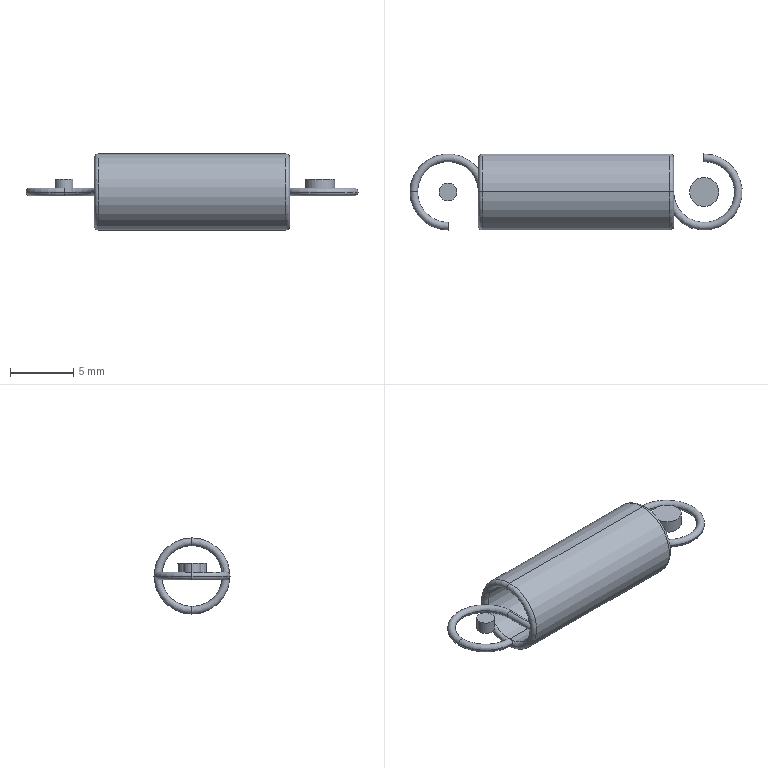Part | STEP file | 11-AWY6_2511 | 3 solids | 28 faces | box 26.2 x 6 x 6 mm | volume 169.712 mm3 | cylinder 12 | torus 10 | plane 6 | commonest cylinder face diameters 0.6 x4 1.401 x2 2.296 x2 4.8 x2 6 x2
STEP:
#1=CARTESIAN_POINT('',(23.748,0.,1.));
#2=VERTEX_POINT('',#1);
#3=CARTESIAN_POINT('',(21.452,0.,1.));
#4=VERTEX_POINT('',#3);
#5=CARTESIAN_POINT('',(22.6,0.,1.));
#6=DIRECTION('',(0.,0.,1.));
#7=DIRECTION('',(1.,0.,0.));
#8=AXIS2_PLACEMENT_3D('',#5,#6,#7);
#9=CIRCLE('',#8,1.148);
#10=EDGE_CURVE('',#2,#4,#9,.T.);
#11=ORIENTED_EDGE('',*,*,#10,.F.);
#12=CARTESIAN_POINT('',(23.748,0.,0.));
#13=VERTEX_POINT('',#12);
#14=CARTESIAN_POINT('',(23.748,0.,1.));
#15=DIRECTION('',(0.,0.,-1.));
#16=VECTOR('',#15,1000.);
#17=LINE('',#14,#16);
#18=EDGE_CURVE('',#2,#13,#17,.T.);
#19=ORIENTED_EDGE('',*,*,#18,.T.);
#20=CARTESIAN_POINT('',(21.452,0.,0.));
#21=VERTEX_POINT('',#20);
#22=CARTESIAN_POINT('',(22.6,0.,0.));
#23=DIRECTION('',(0.,0.,1.));
#24=DIRECTION('',(1.,0.,0.));
#25=AXIS2_PLACEMENT_3D('',#22,#23,#24);
#26=CIRCLE('',#25,1.148);
#27=EDGE_CURVE('',#13,#21,#26,.T.);
#28=ORIENTED_EDGE('',*,*,#27,.T.);
#29=CARTESIAN_POINT('',(21.452,0.,1.));
#30=DIRECTION('',(0.,0.,-1.));
#31=VECTOR('',#30,1000.);
#32=LINE('',#29,#31);
#33=EDGE_CURVE('',#4,#21,#32,.T.);
#34=ORIENTED_EDGE('',*,*,#33,.F.);
#35=EDGE_LOOP('',(#11,#19,#28,#34));
#36=FACE_OUTER_BOUND('',#35,.T.);
#37=CARTESIAN_POINT('',(22.6,0.,1.));
#38=DIRECTION('',(0.,0.,-1.));
#39=DIRECTION('',(-1.,0.,0.));
#40=AXIS2_PLACEMENT_3D('',#37,#38,#39);
#41=CYLINDRICAL_SURFACE('',#40,1.148);
#42=ADVANCED_FACE('',(#36),#41,.T.);
#43=ORIENTED_EDGE('',*,*,#18,.F.);
#44=CARTESIAN_POINT('',(22.6,0.,1.));
#45=DIRECTION('',(0.,0.,1.));
#46=DIRECTION('',(1.,0.,0.));
#47=AXIS2_PLACEMENT_3D('',#44,#45,#46);
#48=CIRCLE('',#47,1.148);
#49=EDGE_CURVE('',#4,#2,#48,.T.);
#50=ORIENTED_EDGE('',*,*,#49,.F.);
#51=ORIENTED_EDGE('',*,*,#33,.T.);
#52=CARTESIAN_POINT('',(22.6,0.,0.));
#53=DIRECTION('',(0.,0.,1.));
#54=DIRECTION('',(1.,0.,0.));
#55=AXIS2_PLACEMENT_3D('',#52,#53,#54);
#56=CIRCLE('',#55,1.148);
#57=EDGE_CURVE('',#21,#13,#56,.T.);
#58=ORIENTED_EDGE('',*,*,#57,.T.);
#59=EDGE_LOOP('',(#43,#50,#51,#58));
#60=FACE_OUTER_BOUND('',#59,.T.);
#61=CARTESIAN_POINT('',(22.6,0.,1.));
#62=DIRECTION('',(0.,0.,-1.));
#63=DIRECTION('',(-1.,0.,0.));
#64=AXIS2_PLACEMENT_3D('',#61,#62,#63);
#65=CYLINDRICAL_SURFACE('',#64,1.148);
#66=ADVANCED_FACE('',(#60),#65,.T.);
#67=ORIENTED_EDGE('',*,*,#49,.T.);
#68=ORIENTED_EDGE('',*,*,#10,.T.);
#69=EDGE_LOOP('',(#67,#68));
#70=FACE_OUTER_BOUND('',#69,.T.);
#71=CARTESIAN_POINT('',(22.6,0.,1.));
#72=DIRECTION('',(0.,0.,1.));
#73=DIRECTION('',(1.,0.,0.));
#74=AXIS2_PLACEMENT_3D('',#71,#72,#73);
#75=PLANE('',#74);
#76=ADVANCED_FACE('',(#70),#75,.T.);
#77=ORIENTED_EDGE('',*,*,#57,.F.);
#78=ORIENTED_EDGE('',*,*,#27,.F.);
#79=EDGE_LOOP('',(#77,#78));
#80=FACE_OUTER_BOUND('',#79,.T.);
#81=CARTESIAN_POINT('',(22.6,0.,0.));
#82=DIRECTION('',(0.,0.,1.));
#83=DIRECTION('',(1.,0.,0.));
#84=AXIS2_PLACEMENT_3D('',#81,#82,#83);
#85=PLANE('',#84);
#86=ADVANCED_FACE('',(#80),#85,.F.);
#87=CLOSED_SHELL('',(#42,#66,#76,#86));
#88=MANIFOLD_SOLID_BREP('',#87);
#89=CARTESIAN_POINT('',(3.1,0.,1.));
#90=VERTEX_POINT('',#89);
#91=CARTESIAN_POINT('',(1.7,0.,1.));
#92=VERTEX_POINT('',#91);
#93=CARTESIAN_POINT('',(2.4,0.,1.));
#94=DIRECTION('',(0.,0.,1.));
#95=DIRECTION('',(1.,0.,0.));
#96=AXIS2_PLACEMENT_3D('',#93,#94,#95);
#97=CIRCLE('',#96,0.7003);
#98=EDGE_CURVE('',#90,#92,#97,.T.);
#99=ORIENTED_EDGE('',*,*,#98,.F.);
#100=CARTESIAN_POINT('',(3.1,0.,0.));
#101=VERTEX_POINT('',#100);
#102=CARTESIAN_POINT('',(3.1,0.,1.));
#103=DIRECTION('',(0.,0.,-1.));
#104=VECTOR('',#103,1000.);
#105=LINE('',#102,#104);
#106=EDGE_CURVE('',#90,#101,#105,.T.);
#107=ORIENTED_EDGE('',*,*,#106,.T.);
#108=CARTESIAN_POINT('',(1.7,0.,0.));
#109=VERTEX_POINT('',#108);
#110=CARTESIAN_POINT('',(2.4,0.,0.));
#111=DIRECTION('',(0.,0.,1.));
#112=DIRECTION('',(1.,0.,0.));
#113=AXIS2_PLACEMENT_3D('',#110,#111,#112);
#114=CIRCLE('',#113,0.7003);
#115=EDGE_CURVE('',#101,#109,#114,.T.);
#116=ORIENTED_EDGE('',*,*,#115,.T.);
#117=CARTESIAN_POINT('',(1.7,0.,1.));
#118=DIRECTION('',(0.,0.,-1.));
#119=VECTOR('',#118,1000.);
#120=LINE('',#117,#119);
#121=EDGE_CURVE('',#92,#109,#120,.T.);
#122=ORIENTED_EDGE('',*,*,#121,.F.);
#123=EDGE_LOOP('',(#99,#107,#116,#122));
#124=FACE_OUTER_BOUND('',#123,.T.);
#125=CARTESIAN_POINT('',(2.4,0.,1.));
#126=DIRECTION('',(0.,0.,-1.));
#127=DIRECTION('',(-1.,0.,0.));
#128=AXIS2_PLACEMENT_3D('',#125,#126,#127);
#129=CYLINDRICAL_SURFACE('',#128,0.7003);
#130=ADVANCED_FACE('',(#124),#129,.T.);
#131=ORIENTED_EDGE('',*,*,#106,.F.);
#132=CARTESIAN_POINT('',(2.4,0.,1.));
#133=DIRECTION('',(0.,0.,1.));
#134=DIRECTION('',(1.,0.,0.));
#135=AXIS2_PLACEMENT_3D('',#132,#133,#134);
#136=CIRCLE('',#135,0.7003);
#137=EDGE_CURVE('',#92,#90,#136,.T.);
#138=ORIENTED_EDGE('',*,*,#137,.F.);
#139=ORIENTED_EDGE('',*,*,#121,.T.);
#140=CARTESIAN_POINT('',(2.4,0.,0.));
#141=DIRECTION('',(0.,0.,1.));
#142=DIRECTION('',(1.,0.,0.));
#143=AXIS2_PLACEMENT_3D('',#140,#141,#142);
#144=CIRCLE('',#143,0.7003);
#145=EDGE_CURVE('',#109,#101,#144,.T.);
#146=ORIENTED_EDGE('',*,*,#145,.T.);
#147=EDGE_LOOP('',(#131,#138,#139,#146));
#148=FACE_OUTER_BOUND('',#147,.T.);
#149=CARTESIAN_POINT('',(2.4,0.,1.));
#150=DIRECTION('',(0.,0.,-1.));
#151=DIRECTION('',(-1.,0.,0.));
#152=AXIS2_PLACEMENT_3D('',#149,#150,#151);
#153=CYLINDRICAL_SURFACE('',#152,0.7003);
#154=ADVANCED_FACE('',(#148),#153,.T.);
#155=ORIENTED_EDGE('',*,*,#137,.T.);
#156=ORIENTED_EDGE('',*,*,#98,.T.);
#157=EDGE_LOOP('',(#155,#156));
#158=FACE_OUTER_BOUND('',#157,.T.);
#159=CARTESIAN_POINT('',(2.4,0.,1.));
#160=DIRECTION('',(0.,0.,1.));
#161=DIRECTION('',(1.,0.,0.));
#162=AXIS2_PLACEMENT_3D('',#159,#160,#161);
#163=PLANE('',#162);
#164=ADVANCED_FACE('',(#158),#163,.T.);
#165=ORIENTED_EDGE('',*,*,#145,.F.);
#166=ORIENTED_EDGE('',*,*,#115,.F.);
#167=EDGE_LOOP('',(#165,#166));
#168=FACE_OUTER_BOUND('',#167,.T.);
#169=CARTESIAN_POINT('',(2.4,0.,0.));
#170=DIRECTION('',(0.,0.,1.));
#171=DIRECTION('',(1.,0.,0.));
#172=AXIS2_PLACEMENT_3D('',#169,#170,#171);
#173=PLANE('',#172);
#174=ADVANCED_FACE('',(#168),#173,.F.);
#175=CLOSED_SHELL('',(#130,#154,#164,#174));
#176=MANIFOLD_SOLID_BREP('',#175);
#177=CARTESIAN_POINT('',(-0.6,0.,0.));
#178=VERTEX_POINT('',#177);
#179=CARTESIAN_POINT('',(0.,0.,0.));
#180=VERTEX_POINT('',#179);
#181=CARTESIAN_POINT('',(-0.3,0.,0.));
#182=DIRECTION('',(0.,-1.,0.));
#183=DIRECTION('',(0.,0.,-1.));
#184=AXIS2_PLACEMENT_3D('',#181,#182,#183);
#185=CIRCLE('',#184,0.3);
#186=EDGE_CURVE('',#178,#180,#185,.T.);
#187=ORIENTED_EDGE('',*,*,#186,.F.);
#188=CARTESIAN_POINT('',(5.4,0.,0.));
#189=VERTEX_POINT('',#188);
#190=CARTESIAN_POINT('',(2.4,0.,0.));
#191=DIRECTION('',(0.,0.,-1.));
#192=DIRECTION('',(-1.,0.,0.));
#193=AXIS2_PLACEMENT_3D('',#190,#191,#192);
#194=CIRCLE('',#193,3.);
#195=EDGE_CURVE('',#178,#189,#194,.T.);
#196=ORIENTED_EDGE('',*,*,#195,.T.);
#197=CARTESIAN_POINT('',(5.1,0.,-0.3));
#198=VERTEX_POINT('',#197);
#199=CARTESIAN_POINT('',(5.1,0.,0.));
#200=DIRECTION('',(0.,-1.,0.));
#201=DIRECTION('',(0.,0.,-1.));
#202=AXIS2_PLACEMENT_3D('',#199,#200,#201);
#203=CIRCLE('',#202,0.3);
#204=EDGE_CURVE('',#198,#189,#203,.T.);
#205=ORIENTED_EDGE('',*,*,#204,.F.);
#206=CARTESIAN_POINT('',(4.8,0.,0.));
#207=VERTEX_POINT('',#206);
#208=CARTESIAN_POINT('',(5.1,0.,0.));
#209=DIRECTION('',(0.,-1.,0.));
#210=DIRECTION('',(0.,0.,-1.));
#211=AXIS2_PLACEMENT_3D('',#208,#209,#210);
#212=CIRCLE('',#211,0.3);
#213=EDGE_CURVE('',#207,#198,#212,.T.);
#214=ORIENTED_EDGE('',*,*,#213,.F.);
#215=CARTESIAN_POINT('',(2.4,0.,0.));
#216=DIRECTION('',(0.,0.,-1.));
#217=DIRECTION('',(-1.,0.,0.));
#218=AXIS2_PLACEMENT_3D('',#215,#216,#217);
#219=CIRCLE('',#218,2.4);
#220=EDGE_CURVE('',#180,#207,#219,.T.);
#221=ORIENTED_EDGE('',*,*,#220,.F.);
#222=EDGE_LOOP('',(#187,#196,#205,#214,#221));
#223=FACE_OUTER_BOUND('',#222,.T.);
#224=CARTESIAN_POINT('',(2.4,0.,0.));
#225=DIRECTION('',(0.,0.,-1.));
#226=DIRECTION('',(-1.,0.,0.));
#227=AXIS2_PLACEMENT_3D('',#224,#225,#226);
#228=TOROIDAL_SURFACE('',#227,2.7,0.3);
#229=ADVANCED_FACE('',(#223),#228,.T.);
#230=CARTESIAN_POINT('',(22.558,2.4,0.));
#231=VERTEX_POINT('',#230);
#232=CARTESIAN_POINT('',(22.548,3.,0.));
#233=VERTEX_POINT('',#232);
#234=CARTESIAN_POINT('',(22.553,2.7,0.));
#235=DIRECTION('',(0.9998,0.01745,0.));
#236=DIRECTION('',(0.,0.,1.));
#237=AXIS2_PLACEMENT_3D('',#234,#235,#236);
#238=CIRCLE('',#237,0.3);
#239=EDGE_CURVE('',#231,#233,#238,.T.);
#240=ORIENTED_EDGE('',*,*,#239,.T.);
#241=CARTESIAN_POINT('',(19.6,0.,0.));
#242=VERTEX_POINT('',#241);
#243=CARTESIAN_POINT('',(22.6,0.,0.));
#244=DIRECTION('',(0.,0.,-1.));
#245=DIRECTION('',(-1.,0.,0.));
#246=AXIS2_PLACEMENT_3D('',#243,#244,#245);
#247=CIRCLE('',#246,3.);
#248=EDGE_CURVE('',#233,#242,#247,.T.);
#249=ORIENTED_EDGE('',*,*,#248,.T.);
#250=CARTESIAN_POINT('',(19.9,0.,-0.3));
#251=VERTEX_POINT('',#250);
#252=CARTESIAN_POINT('',(19.9,0.,0.));
#253=DIRECTION('',(0.,1.,0.));
#254=DIRECTION('',(0.,0.,1.));
#255=AXIS2_PLACEMENT_3D('',#252,#253,#254);
#256=CIRCLE('',#255,0.3);
#257=EDGE_CURVE('',#251,#242,#256,.T.);
#258=ORIENTED_EDGE('',*,*,#257,.F.);
#259=CARTESIAN_POINT('',(20.2,0.,0.));
#260=VERTEX_POINT('',#259);
#261=CARTESIAN_POINT('',(19.9,0.,0.));
#262=DIRECTION('',(0.,1.,0.));
#263=DIRECTION('',(0.,0.,1.));
#264=AXIS2_PLACEMENT_3D('',#261,#262,#263);
#265=CIRCLE('',#264,0.3);
#266=EDGE_CURVE('',#260,#251,#265,.T.);
#267=ORIENTED_EDGE('',*,*,#266,.F.);
#268=CARTESIAN_POINT('',(22.6,0.,0.));
#269=DIRECTION('',(0.,0.,-1.));
#270=DIRECTION('',(-1.,0.,0.));
#271=AXIS2_PLACEMENT_3D('',#268,#269,#270);
#272=CIRCLE('',#271,2.4);
#273=EDGE_CURVE('',#231,#260,#272,.T.);
#274=ORIENTED_EDGE('',*,*,#273,.F.);
#275=EDGE_LOOP('',(#240,#249,#258,#267,#274));
#276=FACE_OUTER_BOUND('',#275,.T.);
#277=CARTESIAN_POINT('',(22.6,0.,0.));
#278=DIRECTION('',(0.,0.,-1.));
#279=DIRECTION('',(-1.,0.,0.));
#280=AXIS2_PLACEMENT_3D('',#277,#278,#279);
#281=TOROIDAL_SURFACE('',#280,2.7,0.3);
#282=ADVANCED_FACE('',(#276),#281,.T.);
#283=CARTESIAN_POINT('',(2.452,-3.,0.));
#284=VERTEX_POINT('',#283);
#285=CARTESIAN_POINT('',(2.442,-2.4,0.));
#286=VERTEX_POINT('',#285);
#287=CARTESIAN_POINT('',(2.447,-2.7,0.));
#288=DIRECTION('',(0.9998,0.01745,0.));
#289=DIRECTION('',(0.,0.,1.));
#290=AXIS2_PLACEMENT_3D('',#287,#288,#289);
#291=CIRCLE('',#290,0.3);
#292=EDGE_CURVE('',#284,#286,#291,.T.);
#293=ORIENTED_EDGE('',*,*,#292,.F.);
#294=CARTESIAN_POINT('',(2.4,0.,0.));
#295=DIRECTION('',(0.,0.,-1.));
#296=DIRECTION('',(-1.,0.,0.));
#297=AXIS2_PLACEMENT_3D('',#294,#295,#296);
#298=CIRCLE('',#297,3.);
#299=EDGE_CURVE('',#284,#178,#298,.T.);
#300=ORIENTED_EDGE('',*,*,#299,.T.);
#301=ORIENTED_EDGE('',*,*,#186,.T.);
#302=CARTESIAN_POINT('',(2.4,0.,0.));
#303=DIRECTION('',(0.,0.,-1.));
#304=DIRECTION('',(-1.,0.,0.));
#305=AXIS2_PLACEMENT_3D('',#302,#303,#304);
#306=CIRCLE('',#305,2.4);
#307=EDGE_CURVE('',#286,#180,#306,.T.);
#308=ORIENTED_EDGE('',*,*,#307,.F.);
#309=EDGE_LOOP('',(#293,#300,#301,#308));
#310=FACE_OUTER_BOUND('',#309,.T.);
#311=CARTESIAN_POINT('',(2.4,0.,0.));
#312=DIRECTION('',(0.,0.,-1.));
#313=DIRECTION('',(-1.,0.,0.));
#314=AXIS2_PLACEMENT_3D('',#311,#312,#313);
#315=TOROIDAL_SURFACE('',#314,2.7,0.3);
#316=ADVANCED_FACE('',(#310),#315,.T.);
#317=ORIENTED_EDGE('',*,*,#299,.F.);
#318=CARTESIAN_POINT('',(2.447,-2.7,0.));
#319=DIRECTION('',(0.9998,0.01745,0.));
#320=DIRECTION('',(0.,0.,1.));
#321=AXIS2_PLACEMENT_3D('',#318,#319,#320);
#322=CIRCLE('',#321,0.3);
#323=EDGE_CURVE('',#286,#284,#322,.T.);
#324=ORIENTED_EDGE('',*,*,#323,.F.);
#325=ORIENTED_EDGE('',*,*,#307,.T.);
#326=CARTESIAN_POINT('',(-0.3,0.,0.));
#327=DIRECTION('',(0.,-1.,0.));
#328=DIRECTION('',(0.,0.,-1.));
#329=AXIS2_PLACEMENT_3D('',#326,#327,#328);
#330=CIRCLE('',#329,0.3);
#331=EDGE_CURVE('',#180,#178,#330,.T.);
#332=ORIENTED_EDGE('',*,*,#331,.T.);
#333=EDGE_LOOP('',(#317,#324,#325,#332));
#334=FACE_OUTER_BOUND('',#333,.T.);
#335=CARTESIAN_POINT('',(2.4,0.,0.));
#336=DIRECTION('',(0.,0.,-1.));
#337=DIRECTION('',(-1.,0.,0.));
#338=AXIS2_PLACEMENT_3D('',#335,#336,#337);
#339=TOROIDAL_SURFACE('',#338,2.7,0.3);
#340=ADVANCED_FACE('',(#334),#339,.T.);
#341=ORIENTED_EDGE('',*,*,#204,.T.);
#342=CARTESIAN_POINT('',(5.1,0.,0.3));
#343=VERTEX_POINT('',#342);
#344=CARTESIAN_POINT('',(5.1,0.,0.));
#345=DIRECTION('',(0.,-1.,0.));
#346=DIRECTION('',(0.,0.,-1.));
#347=AXIS2_PLACEMENT_3D('',#344,#345,#346);
#348=CIRCLE('',#347,0.3);
#349=EDGE_CURVE('',#189,#343,#348,.T.);
#350=ORIENTED_EDGE('',*,*,#349,.T.);
#351=CARTESIAN_POINT('',(5.1,-2.381,0.3));
#352=VERTEX_POINT('',#351);
#353=CARTESIAN_POINT('',(5.1,-2.7,0.3));
#354=DIRECTION('',(0.,-1.,0.));
#355=VECTOR('',#354,1000.);
#356=LINE('',#353,#355);
#357=EDGE_CURVE('',#343,#352,#356,.T.);
#358=ORIENTED_EDGE('',*,*,#357,.T.);
#359=CARTESIAN_POINT('',(5.1,-2.381,-0.3));
#360=VERTEX_POINT('',#359);
#361=CARTESIAN_POINT('',(5.1,-2.381,-0.3));
#362=CARTESIAN_POINT('',(5.179,-2.381,-0.3));
#363=CARTESIAN_POINT('',(5.257,-2.386,-0.2674));
#364=CARTESIAN_POINT('',(5.367,-2.396,-0.1568));
#365=CARTESIAN_POINT('',(5.4,-2.4,-0.07846));
#366=CARTESIAN_POINT('',(5.4,-2.4,0.07824));
#367=CARTESIAN_POINT('',(5.368,-2.396,0.1561));
#368=CARTESIAN_POINT('',(5.256,-2.386,0.2681));
#369=CARTESIAN_POINT('',(5.178,-2.381,0.3));
#370=CARTESIAN_POINT('',(5.1,-2.381,0.3));
#371=B_SPLINE_CURVE_WITH_KNOTS('',3,(#361,#362,#363,#364,#365,#366,#367,#368,#369,#370),.UNSPECIFIED.,.F.,.F.,(4,2,2,2,4),(0.,0.0002347,0.0004694,0.0007041,0.0009389),.UNSPECIFIED.);
#372=EDGE_CURVE('',#360,#352,#371,.T.);
#373=ORIENTED_EDGE('',*,*,#372,.F.);
#374=CARTESIAN_POINT('',(5.1,-2.7,-0.3));
#375=DIRECTION('',(0.,-1.,0.));
#376=VECTOR('',#375,1000.);
#377=LINE('',#374,#376);
#378=EDGE_CURVE('',#198,#360,#377,.T.);
#379=ORIENTED_EDGE('',*,*,#378,.F.);
#380=EDGE_LOOP('',(#341,#350,#358,#373,#379));
#381=FACE_OUTER_BOUND('',#380,.T.);
#382=CARTESIAN_POINT('',(5.1,-2.7,0.));
#383=DIRECTION('',(0.,-1.,0.));
#384=DIRECTION('',(0.,0.,-1.));
#385=AXIS2_PLACEMENT_3D('',#382,#383,#384);
#386=CYLINDRICAL_SURFACE('',#385,0.3);
#387=ADVANCED_FACE('',(#381),#386,.T.);
#388=CARTESIAN_POINT('',(19.9,0.,0.3));
#389=VERTEX_POINT('',#388);
#390=CARTESIAN_POINT('',(19.9,0.,0.));
#391=DIRECTION('',(0.,1.,0.));
#392=DIRECTION('',(0.,0.,1.));
#393=AXIS2_PLACEMENT_3D('',#390,#391,#392);
#394=CIRCLE('',#393,0.3);
#395=EDGE_CURVE('',#389,#260,#394,.T.);
#396=ORIENTED_EDGE('',*,*,#395,.T.);
#397=ORIENTED_EDGE('',*,*,#266,.T.);
#398=CARTESIAN_POINT('',(19.9,2.381,-0.3));
#399=VERTEX_POINT('',#398);
#400=CARTESIAN_POINT('',(19.9,0.,-0.3));
#401=DIRECTION('',(0.,1.,0.));
#402=VECTOR('',#401,1000.);
#403=LINE('',#400,#402);
#404=EDGE_CURVE('',#251,#399,#403,.T.);
#405=ORIENTED_EDGE('',*,*,#404,.T.);
#406=CARTESIAN_POINT('',(20.2,2.7,0.));
#407=VERTEX_POINT('',#406);
#408=CARTESIAN_POINT('',(19.9,2.381,-0.3));
#409=CARTESIAN_POINT('',(19.949,2.381,-0.3));
#410=CARTESIAN_POINT('',(19.996,2.395,-0.2875));
#411=CARTESIAN_POINT('',(20.074,2.439,-0.2481));
#412=CARTESIAN_POINT('',(20.105,2.468,-0.2221));
#413=CARTESIAN_POINT('',(20.178,2.561,-0.1362));
#414=CARTESIAN_POINT('',(20.2,2.632,-0.06843));
#415=CARTESIAN_POINT('',(20.2,2.7,0.));
#416=B_SPLINE_CURVE_WITH_KNOTS('',3,(#408,#409,#410,#411,#412,#413,#414,#415),.UNSPECIFIED.,.F.,.F.,(4,2,2,4),(0.000000196,0.0001454,0.0002906,0.000581),.UNSPECIFIED.);
#417=EDGE_CURVE('',#399,#407,#416,.T.);
#418=ORIENTED_EDGE('',*,*,#417,.T.);
#419=CARTESIAN_POINT('',(19.9,2.381,0.3));
#420=VERTEX_POINT('',#419);
#421=CARTESIAN_POINT('',(20.2,2.7,0.));
#422=CARTESIAN_POINT('',(20.2,2.632,0.0681));
#423=CARTESIAN_POINT('',(20.178,2.561,0.1362));
#424=CARTESIAN_POINT('',(20.105,2.468,0.2218));
#425=CARTESIAN_POINT('',(20.074,2.44,0.2479));
#426=CARTESIAN_POINT('',(19.997,2.396,0.2873));
#427=CARTESIAN_POINT('',(19.949,2.381,0.3));
#428=CARTESIAN_POINT('',(19.9,2.381,0.3));
#429=B_SPLINE_CURVE_WITH_KNOTS('',3,(#421,#422,#423,#424,#425,#426,#427,#428),.UNSPECIFIED.,.F.,.F.,(4,2,2,4),(-0.000003464,0.0002855,0.00043,0.0005745),.UNSPECIFIED.);
#430=EDGE_CURVE('',#407,#420,#429,.T.);
#431=ORIENTED_EDGE('',*,*,#430,.T.);
#432=CARTESIAN_POINT('',(19.9,0.,0.3));
#433=DIRECTION('',(0.,1.,0.));
#434=VECTOR('',#433,1000.);
#435=LINE('',#432,#434);
#436=EDGE_CURVE('',#389,#420,#435,.T.);
#437=ORIENTED_EDGE('',*,*,#436,.F.);
#438=EDGE_LOOP('',(#396,#397,#405,#418,#431,#437));
#439=FACE_OUTER_BOUND('',#438,.T.);
#440=CARTESIAN_POINT('',(19.9,0.,0.));
#441=DIRECTION('',(0.,1.,0.));
#442=DIRECTION('',(0.,0.,1.));
#443=AXIS2_PLACEMENT_3D('',#440,#441,#442);
#444=CYLINDRICAL_SURFACE('',#443,0.3);
#445=ADVANCED_FACE('',(#439),#444,.T.);
#446=CARTESIAN_POINT('',(19.9,0.,3.));
#447=VERTEX_POINT('',#446);
#448=CARTESIAN_POINT('',(19.9,0.,-3.));
#449=VERTEX_POINT('',#448);
#450=CARTESIAN_POINT('',(19.9,0.,0.));
#451=DIRECTION('',(-1.,0.,0.));
#452=DIRECTION('',(0.,0.,1.));
#453=AXIS2_PLACEMENT_3D('',#450,#451,#452);
#454=CIRCLE('',#453,3.);
#455=EDGE_CURVE('',#447,#449,#454,.T.);
#456=ORIENTED_EDGE('',*,*,#455,.T.);
#457=CARTESIAN_POINT('',(5.1,0.,-3.));
#458=VERTEX_POINT('',#457);
#459=CARTESIAN_POINT('',(20.2,0.,-3.));
#460=DIRECTION('',(-1.,0.,0.));
#461=VECTOR('',#460,1000.);
#462=LINE('',#459,#461);
#463=EDGE_CURVE('',#449,#458,#462,.T.);
#464=ORIENTED_EDGE('',*,*,#463,.T.);
#465=CARTESIAN_POINT('',(5.1,0.,3.));
#466=VERTEX_POINT('',#465);
#467=CARTESIAN_POINT('',(5.1,0.,0.));
#468=DIRECTION('',(-1.,0.,0.));
#469=DIRECTION('',(0.,0.,1.));
#470=AXIS2_PLACEMENT_3D('',#467,#468,#469);
#471=CIRCLE('',#470,3.);
#472=EDGE_CURVE('',#466,#458,#471,.T.);
#473=ORIENTED_EDGE('',*,*,#472,.F.);
#474=CARTESIAN_POINT('',(20.2,0.,3.));
#475=DIRECTION('',(-1.,0.,0.));
#476=VECTOR('',#475,1000.);
#477=LINE('',#474,#476);
#478=EDGE_CURVE('',#447,#466,#477,.T.);
#479=ORIENTED_EDGE('',*,*,#478,.F.);
#480=EDGE_LOOP('',(#456,#464,#473,#479));
#481=FACE_OUTER_BOUND('',#480,.T.);
#482=CARTESIAN_POINT('',(20.2,0.,0.));
#483=DIRECTION('',(-1.,0.,0.));
#484=DIRECTION('',(0.,0.,1.));
#485=AXIS2_PLACEMENT_3D('',#482,#483,#484);
#486=CYLINDRICAL_SURFACE('',#485,3.);
#487=ADVANCED_FACE('',(#481),#486,.T.);
#488=ORIENTED_EDGE('',*,*,#472,.T.);
#489=CARTESIAN_POINT('',(5.1,0.,-2.4));
#490=VERTEX_POINT('',#489);
#491=CARTESIAN_POINT('',(5.1,0.,-2.7));
#492=DIRECTION('',(0.,1.,0.));
#493=DIRECTION('',(0.,0.,1.));
#494=AXIS2_PLACEMENT_3D('',#491,#492,#493);
#495=CIRCLE('',#494,0.3);
#496=EDGE_CURVE('',#458,#490,#495,.T.);
#497=ORIENTED_EDGE('',*,*,#496,.T.);
#498=CARTESIAN_POINT('',(5.1,0.,2.4));
#499=VERTEX_POINT('',#498);
#500=CARTESIAN_POINT('',(5.1,0.,0.));
#501=DIRECTION('',(-1.,0.,0.));
#502=DIRECTION('',(0.,0.,1.));
#503=AXIS2_PLACEMENT_3D('',#500,#501,#502);
#504=CIRCLE('',#503,2.4);
#505=EDGE_CURVE('',#499,#490,#504,.T.);
#506=ORIENTED_EDGE('',*,*,#505,.F.);
#507=CARTESIAN_POINT('',(5.1,0.,2.7));
#508=DIRECTION('',(0.,-1.,0.));
#509=DIRECTION('',(0.,0.,-1.));
#510=AXIS2_PLACEMENT_3D('',#507,#508,#509);
#511=CIRCLE('',#510,0.3);
#512=EDGE_CURVE('',#466,#499,#511,.T.);
#513=ORIENTED_EDGE('',*,*,#512,.F.);
#514=EDGE_LOOP('',(#488,#497,#506,#513));
#515=FACE_OUTER_BOUND('',#514,.T.);
#516=CARTESIAN_POINT('',(5.1,0.,0.));
#517=DIRECTION('',(-1.,0.,0.));
#518=DIRECTION('',(0.,0.,1.));
#519=AXIS2_PLACEMENT_3D('',#516,#517,#518);
#520=TOROIDAL_SURFACE('',#519,2.7,0.3);
#521=ADVANCED_FACE('',(#515),#520,.T.);
#522=CARTESIAN_POINT('',(19.9,0.,-2.4));
#523=VERTEX_POINT('',#522);
#524=CARTESIAN_POINT('',(19.9,0.,0.));
#525=DIRECTION('',(-1.,0.,0.));
#526=DIRECTION('',(0.,0.,1.));
#527=AXIS2_PLACEMENT_3D('',#524,#525,#526);
#528=CIRCLE('',#527,2.4);
#529=EDGE_CURVE('',#399,#523,#528,.T.);
#530=ORIENTED_EDGE('',*,*,#529,.T.);
#531=CARTESIAN_POINT('',(19.9,0.,-2.7));
#532=DIRECTION('',(0.,1.,0.));
#533=DIRECTION('',(0.,0.,1.));
#534=AXIS2_PLACEMENT_3D('',#531,#532,#533);
#535=CIRCLE('',#534,0.3);
#536=EDGE_CURVE('',#523,#449,#535,.T.);
#537=ORIENTED_EDGE('',*,*,#536,.T.);
#538=ORIENTED_EDGE('',*,*,#455,.F.);
#539=CARTESIAN_POINT('',(19.9,0.,2.4));
#540=VERTEX_POINT('',#539);
#541=CARTESIAN_POINT('',(19.9,0.,2.7));
#542=DIRECTION('',(0.,-1.,0.));
#543=DIRECTION('',(0.,0.,-1.));
#544=AXIS2_PLACEMENT_3D('',#541,#542,#543);
#545=CIRCLE('',#544,0.3);
#546=EDGE_CURVE('',#540,#447,#545,.T.);
#547=ORIENTED_EDGE('',*,*,#546,.F.);
#548=CARTESIAN_POINT('',(19.9,0.,0.));
#549=DIRECTION('',(-1.,0.,0.));
#550=DIRECTION('',(0.,0.,1.));
#551=AXIS2_PLACEMENT_3D('',#548,#549,#550);
#552=CIRCLE('',#551,2.4);
#553=EDGE_CURVE('',#540,#420,#552,.T.);
#554=ORIENTED_EDGE('',*,*,#553,.T.);
#555=ORIENTED_EDGE('',*,*,#430,.F.);
#556=ORIENTED_EDGE('',*,*,#417,.F.);
#557=EDGE_LOOP('',(#530,#537,#538,#547,#554,#555,#556));
#558=FACE_OUTER_BOUND('',#557,.T.);
#559=CARTESIAN_POINT('',(19.9,0.,0.));
#560=DIRECTION('',(-1.,0.,0.));
#561=DIRECTION('',(0.,0.,1.));
#562=AXIS2_PLACEMENT_3D('',#559,#560,#561);
#563=TOROIDAL_SURFACE('',#562,2.7,0.3);
#564=ADVANCED_FACE('',(#558),#563,.T.);
#565=CARTESIAN_POINT('',(19.9,0.,0.));
#566=DIRECTION('',(-1.,0.,0.));
#567=DIRECTION('',(0.,0.,1.));
#568=AXIS2_PLACEMENT_3D('',#565,#566,#567);
#569=CIRCLE('',#568,2.4);
#570=EDGE_CURVE('',#523,#540,#569,.T.);
#571=ORIENTED_EDGE('',*,*,#570,.F.);
#572=CARTESIAN_POINT('',(20.2,0.,-2.4));
#573=DIRECTION('',(-1.,0.,0.));
#574=VECTOR('',#573,1000.);
#575=LINE('',#572,#574);
#576=EDGE_CURVE('',#523,#490,#575,.T.);
#577=ORIENTED_EDGE('',*,*,#576,.T.);
#578=CARTESIAN_POINT('',(5.1,0.,0.));
#579=DIRECTION('',(-1.,0.,0.));
#580=DIRECTION('',(0.,0.,1.));
#581=AXIS2_PLACEMENT_3D('',#578,#579,#580);
#582=CIRCLE('',#581,2.4);
#583=EDGE_CURVE('',#490,#360,#582,.T.);
#584=ORIENTED_EDGE('',*,*,#583,.T.);
#585=ORIENTED_EDGE('',*,*,#372,.T.);
#586=CARTESIAN_POINT('',(5.1,0.,0.));
#587=DIRECTION('',(-1.,0.,0.));
#588=DIRECTION('',(0.,0.,1.));
#589=AXIS2_PLACEMENT_3D('',#586,#587,#588);
#590=CIRCLE('',#589,2.4);
#591=EDGE_CURVE('',#352,#499,#590,.T.);
#592=ORIENTED_EDGE('',*,*,#591,.T.);
#593=CARTESIAN_POINT('',(20.2,0.,2.4));
#594=DIRECTION('',(-1.,0.,0.));
#595=VECTOR('',#594,1000.);
#596=LINE('',#593,#595);
#597=EDGE_CURVE('',#540,#499,#596,.T.);
#598=ORIENTED_EDGE('',*,*,#597,.F.);
#599=EDGE_LOOP('',(#571,#577,#584,#585,#592,#598));
#600=FACE_OUTER_BOUND('',#599,.T.);
#601=CARTESIAN_POINT('',(20.2,0.,0.));
#602=DIRECTION('',(-1.,0.,0.));
#603=DIRECTION('',(0.,0.,1.));
#604=AXIS2_PLACEMENT_3D('',#601,#602,#603);
#605=CYLINDRICAL_SURFACE('',#604,2.4);
#606=ADVANCED_FACE('',(#600),#605,.F.);
#607=ORIENTED_EDGE('',*,*,#576,.F.);
#608=ORIENTED_EDGE('',*,*,#529,.F.);
#609=CARTESIAN_POINT('',(19.9,2.381,0.3));
#610=CARTESIAN_POINT('',(19.821,2.381,0.3));
#611=CARTESIAN_POINT('',(19.743,2.386,0.2674));
#612=CARTESIAN_POINT('',(19.633,2.396,0.1568));
#613=CARTESIAN_POINT('',(19.6,2.4,0.07846));
#614=CARTESIAN_POINT('',(19.6,2.4,-0.07824));
#615=CARTESIAN_POINT('',(19.632,2.396,-0.1561));
#616=CARTESIAN_POINT('',(19.744,2.386,-0.2681));
#617=CARTESIAN_POINT('',(19.822,2.381,-0.3));
#618=CARTESIAN_POINT('',(19.9,2.381,-0.3));
#619=B_SPLINE_CURVE_WITH_KNOTS('',3,(#609,#610,#611,#612,#613,#614,#615,#616,#617,#618),.UNSPECIFIED.,.F.,.F.,(4,2,2,2,4),(0.,0.0002347,0.0004694,0.0007041,0.0009389),.UNSPECIFIED.);
#620=EDGE_CURVE('',#420,#399,#619,.T.);
#621=ORIENTED_EDGE('',*,*,#620,.F.);
#622=ORIENTED_EDGE('',*,*,#553,.F.);
#623=ORIENTED_EDGE('',*,*,#597,.T.);
#624=ORIENTED_EDGE('',*,*,#505,.T.);
#625=EDGE_LOOP('',(#607,#608,#621,#622,#623,#624));
#626=FACE_OUTER_BOUND('',#625,.T.);
#627=CARTESIAN_POINT('',(20.2,0.,0.));
#628=DIRECTION('',(-1.,0.,0.));
#629=DIRECTION('',(0.,0.,1.));
#630=AXIS2_PLACEMENT_3D('',#627,#628,#629);
#631=CYLINDRICAL_SURFACE('',#630,2.4);
#632=ADVANCED_FACE('',(#626),#631,.F.);
#633=ORIENTED_EDGE('',*,*,#536,.F.);
#634=ORIENTED_EDGE('',*,*,#570,.T.);
#635=ORIENTED_EDGE('',*,*,#546,.T.);
#636=CARTESIAN_POINT('',(19.9,0.,0.));
#637=DIRECTION('',(-1.,0.,0.));
#638=DIRECTION('',(0.,0.,1.));
#639=AXIS2_PLACEMENT_3D('',#636,#637,#638);
#640=CIRCLE('',#639,3.);
#641=EDGE_CURVE('',#449,#447,#640,.T.);
#642=ORIENTED_EDGE('',*,*,#641,.F.);
#643=EDGE_LOOP('',(#633,#634,#635,#642));
#644=FACE_OUTER_BOUND('',#643,.T.);
#645=CARTESIAN_POINT('',(19.9,0.,0.));
#646=DIRECTION('',(-1.,0.,0.));
#647=DIRECTION('',(0.,0.,1.));
#648=AXIS2_PLACEMENT_3D('',#645,#646,#647);
#649=TOROIDAL_SURFACE('',#648,2.7,0.3);
#650=ADVANCED_FACE('',(#644),#649,.T.);
#651=ORIENTED_EDGE('',*,*,#496,.F.);
#652=CARTESIAN_POINT('',(5.1,0.,0.));
#653=DIRECTION('',(-1.,0.,0.));
#654=DIRECTION('',(0.,0.,1.));
#655=AXIS2_PLACEMENT_3D('',#652,#653,#654);
#656=CIRCLE('',#655,3.);
#657=EDGE_CURVE('',#458,#466,#656,.T.);
#658=ORIENTED_EDGE('',*,*,#657,.T.);
#659=ORIENTED_EDGE('',*,*,#512,.T.);
#660=ORIENTED_EDGE('',*,*,#591,.F.);
#661=CARTESIAN_POINT('',(4.8,-2.7,0.));
#662=VERTEX_POINT('',#661);
#663=CARTESIAN_POINT('',(5.1,-2.381,0.3));
#664=CARTESIAN_POINT('',(5.051,-2.381,0.3));
#665=CARTESIAN_POINT('',(5.004,-2.395,0.2875));
#666=CARTESIAN_POINT('',(4.926,-2.439,0.2481));
#667=CARTESIAN_POINT('',(4.895,-2.468,0.2221));
#668=CARTESIAN_POINT('',(4.822,-2.561,0.1362));
#669=CARTESIAN_POINT('',(4.8,-2.632,0.06843));
#670=CARTESIAN_POINT('',(4.8,-2.7,0.));
#671=B_SPLINE_CURVE_WITH_KNOTS('',3,(#663,#664,#665,#666,#667,#668,#669,#670),.UNSPECIFIED.,.F.,.F.,(4,2,2,4),(0.000000196,0.0001454,0.0002906,0.000581),.UNSPECIFIED.);
#672=EDGE_CURVE('',#352,#662,#671,.T.);
#673=ORIENTED_EDGE('',*,*,#672,.T.);
#674=CARTESIAN_POINT('',(4.8,-2.7,0.));
#675=CARTESIAN_POINT('',(4.8,-2.632,-0.0681));
#676=CARTESIAN_POINT('',(4.822,-2.561,-0.1362));
#677=CARTESIAN_POINT('',(4.895,-2.468,-0.2218));
#678=CARTESIAN_POINT('',(4.926,-2.44,-0.2479));
#679=CARTESIAN_POINT('',(5.003,-2.396,-0.2873));
#680=CARTESIAN_POINT('',(5.051,-2.381,-0.3));
#681=CARTESIAN_POINT('',(5.1,-2.381,-0.3));
#682=B_SPLINE_CURVE_WITH_KNOTS('',3,(#674,#675,#676,#677,#678,#679,#680,#681),.UNSPECIFIED.,.F.,.F.,(4,2,2,4),(-0.000003464,0.0002855,0.00043,0.0005745),.UNSPECIFIED.);
#683=EDGE_CURVE('',#662,#360,#682,.T.);
#684=ORIENTED_EDGE('',*,*,#683,.T.);
#685=ORIENTED_EDGE('',*,*,#583,.F.);
#686=EDGE_LOOP('',(#651,#658,#659,#660,#673,#684,#685));
#687=FACE_OUTER_BOUND('',#686,.T.);
#688=CARTESIAN_POINT('',(5.1,0.,0.));
#689=DIRECTION('',(-1.,0.,0.));
#690=DIRECTION('',(0.,0.,1.));
#691=AXIS2_PLACEMENT_3D('',#688,#689,#690);
#692=TOROIDAL_SURFACE('',#691,2.7,0.3);
#693=ADVANCED_FACE('',(#687),#692,.T.);
#694=ORIENTED_EDGE('',*,*,#463,.F.);
#695=ORIENTED_EDGE('',*,*,#641,.T.);
#696=ORIENTED_EDGE('',*,*,#478,.T.);
#697=ORIENTED_EDGE('',*,*,#657,.F.);
#698=EDGE_LOOP('',(#694,#695,#696,#697));
#699=FACE_OUTER_BOUND('',#698,.T.);
#700=CARTESIAN_POINT('',(20.2,0.,0.));
#701=DIRECTION('',(-1.,0.,0.));
#702=DIRECTION('',(0.,0.,1.));
#703=AXIS2_PLACEMENT_3D('',#700,#701,#702);
#704=CYLINDRICAL_SURFACE('',#703,3.);
#705=ADVANCED_FACE('',(#699),#704,.T.);
#706=ORIENTED_EDGE('',*,*,#404,.F.);
#707=ORIENTED_EDGE('',*,*,#257,.T.);
#708=CARTESIAN_POINT('',(19.9,0.,0.));
#709=DIRECTION('',(0.,1.,0.));
#710=DIRECTION('',(0.,0.,1.));
#711=AXIS2_PLACEMENT_3D('',#708,#709,#710);
#712=CIRCLE('',#711,0.3);
#713=EDGE_CURVE('',#242,#389,#712,.T.);
#714=ORIENTED_EDGE('',*,*,#713,.T.);
#715=ORIENTED_EDGE('',*,*,#436,.T.);
#716=ORIENTED_EDGE('',*,*,#620,.T.);
#717=EDGE_LOOP('',(#706,#707,#714,#715,#716));
#718=FACE_OUTER_BOUND('',#717,.T.);
#719=CARTESIAN_POINT('',(19.9,0.,0.));
#720=DIRECTION('',(0.,1.,0.));
#721=DIRECTION('',(0.,0.,1.));
#722=AXIS2_PLACEMENT_3D('',#719,#720,#721);
#723=CYLINDRICAL_SURFACE('',#722,0.3);
#724=ADVANCED_FACE('',(#718),#723,.T.);
#725=ORIENTED_EDGE('',*,*,#239,.F.);
#726=CARTESIAN_POINT('',(22.553,2.7,0.));
#727=DIRECTION('',(0.9998,0.01745,0.));
#728=DIRECTION('',(0.,0.,1.));
#729=AXIS2_PLACEMENT_3D('',#726,#727,#728);
#730=CIRCLE('',#729,0.3);
#731=EDGE_CURVE('',#233,#231,#730,.T.);
#732=ORIENTED_EDGE('',*,*,#731,.F.);
#733=EDGE_LOOP('',(#725,#732));
#734=FACE_OUTER_BOUND('',#733,.T.);
#735=CARTESIAN_POINT('',(22.553,2.7,0.));
#736=DIRECTION('',(0.9998,0.01745,0.));
#737=DIRECTION('',(0.,0.,1.));
#738=AXIS2_PLACEMENT_3D('',#735,#736,#737);
#739=PLANE('',#738);
#740=ADVANCED_FACE('',(#734),#739,.F.);
#741=ORIENTED_EDGE('',*,*,#248,.F.);
#742=ORIENTED_EDGE('',*,*,#731,.T.);
#743=ORIENTED_EDGE('',*,*,#273,.T.);
#744=ORIENTED_EDGE('',*,*,#395,.F.);
#745=ORIENTED_EDGE('',*,*,#713,.F.);
#746=EDGE_LOOP('',(#741,#742,#743,#744,#745));
#747=FACE_OUTER_BOUND('',#746,.T.);
#748=CARTESIAN_POINT('',(22.6,0.,0.));
#749=DIRECTION('',(0.,0.,-1.));
#750=DIRECTION('',(-1.,0.,0.));
#751=AXIS2_PLACEMENT_3D('',#748,#749,#750);
#752=TOROIDAL_SURFACE('',#751,2.7,0.3);
#753=ADVANCED_FACE('',(#747),#752,.T.);
#754=ORIENTED_EDGE('',*,*,#357,.F.);
#755=CARTESIAN_POINT('',(5.1,0.,0.));
#756=DIRECTION('',(0.,-1.,0.));
#757=DIRECTION('',(0.,0.,-1.));
#758=AXIS2_PLACEMENT_3D('',#755,#756,#757);
#759=CIRCLE('',#758,0.3);
#760=EDGE_CURVE('',#343,#207,#759,.T.);
#761=ORIENTED_EDGE('',*,*,#760,.T.);
#762=ORIENTED_EDGE('',*,*,#213,.T.);
#763=ORIENTED_EDGE('',*,*,#378,.T.);
#764=ORIENTED_EDGE('',*,*,#683,.F.);
#765=ORIENTED_EDGE('',*,*,#672,.F.);
#766=EDGE_LOOP('',(#754,#761,#762,#763,#764,#765));
#767=FACE_OUTER_BOUND('',#766,.T.);
#768=CARTESIAN_POINT('',(5.1,-2.7,0.));
#769=DIRECTION('',(0.,-1.,0.));
#770=DIRECTION('',(0.,0.,-1.));
#771=AXIS2_PLACEMENT_3D('',#768,#769,#770);
#772=CYLINDRICAL_SURFACE('',#771,0.3);
#773=ADVANCED_FACE('',(#767),#772,.T.);
#774=ORIENTED_EDGE('',*,*,#323,.T.);
#775=ORIENTED_EDGE('',*,*,#292,.T.);
#776=EDGE_LOOP('',(#774,#775));
#777=FACE_OUTER_BOUND('',#776,.T.);
#778=CARTESIAN_POINT('',(2.447,-2.7,0.));
#779=DIRECTION('',(0.9998,0.01745,0.));
#780=DIRECTION('',(0.,0.,1.));
#781=AXIS2_PLACEMENT_3D('',#778,#779,#780);
#782=PLANE('',#781);
#783=ADVANCED_FACE('',(#777),#782,.T.);
#784=ORIENTED_EDGE('',*,*,#195,.F.);
#785=ORIENTED_EDGE('',*,*,#331,.F.);
#786=ORIENTED_EDGE('',*,*,#220,.T.);
#787=ORIENTED_EDGE('',*,*,#760,.F.);
#788=ORIENTED_EDGE('',*,*,#349,.F.);
#789=EDGE_LOOP('',(#784,#785,#786,#787,#788));
#790=FACE_OUTER_BOUND('',#789,.T.);
#791=CARTESIAN_POINT('',(2.4,0.,0.));
#792=DIRECTION('',(0.,0.,-1.));
#793=DIRECTION('',(-1.,0.,0.));
#794=AXIS2_PLACEMENT_3D('',#791,#792,#793);
#795=TOROIDAL_SURFACE('',#794,2.7,0.3);
#796=ADVANCED_FACE('',(#790),#795,.T.);
#797=CLOSED_SHELL('',(#229,#282,#316,#340,#387,#445,#487,#521,#564,#606,#632,#650,#693,#705,#724,#740,#753,#773,#783,#796));
#798=MANIFOLD_SOLID_BREP('',#797);
#799=CARTESIAN_POINT('',(0.,0.,0.));
#800=DIRECTION('',(0.,0.,1.));
#801=DIRECTION('',(1.,0.,0.));
#802=AXIS2_PLACEMENT_3D('',#799,#800,#801);
#803=(LENGTH_UNIT()NAMED_UNIT(*)SI_UNIT(.MILLI.,.METRE.));
#804=UNCERTAINTY_MEASURE_WITH_UNIT(LENGTH_MEASURE(0.00001),#803,'','');
#805=(NAMED_UNIT(*)PLANE_ANGLE_UNIT()SI_UNIT($,.RADIAN.));
#806=(NAMED_UNIT(*)SI_UNIT($,.STERADIAN.)SOLID_ANGLE_UNIT());
#807=(GEOMETRIC_REPRESENTATION_CONTEXT(3)GLOBAL_UNCERTAINTY_ASSIGNED_CONTEXT((#804))GLOBAL_UNIT_ASSIGNED_CONTEXT((#803,#805,#806))REPRESENTATION_CONTEXT('',''));
#808=ADVANCED_BREP_SHAPE_REPRESENTATION('',(#88,#176,#798,#802),#807);